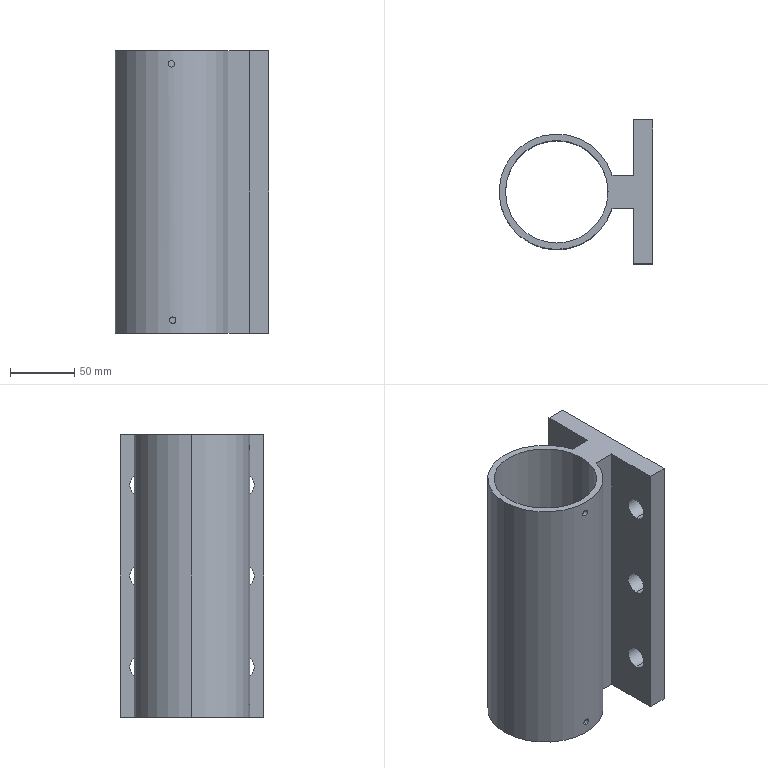Part | SolidWorks | features ICE 2, Extrusion 1 | 1 solid | 29 faces | box 120 x 112 x 220 mm | volume 732141 mm3 | cylinder 20 | plane 9 | commonest cylinder face diameters 17 x12 5 x4 80 x2 90 x2
STEP:
#1=CARTESIAN_POINT('',(0.,-45.,12.5));
#2=VERTEX_POINT('',#1);
#3=CARTESIAN_POINT('',(0.,-45.,7.5));
#4=VERTEX_POINT('',#3);
#5=CARTESIAN_POINT('',(0.,-45.,12.5));
#6=CARTESIAN_POINT('',(-0.1652,-45.,12.5));
#7=CARTESIAN_POINT('',(-0.3277,-44.999,12.484));
#8=CARTESIAN_POINT('',(-0.6473,-44.996,12.42));
#9=CARTESIAN_POINT('',(-0.806,-44.993,12.372));
#10=CARTESIAN_POINT('',(-1.109,-44.987,12.247));
#11=CARTESIAN_POINT('',(-1.252,-44.983,12.17));
#12=CARTESIAN_POINT('',(-1.524,-44.974,11.988));
#13=CARTESIAN_POINT('',(-1.653,-44.97,11.883));
#14=CARTESIAN_POINT('',(-1.883,-44.961,11.652));
#15=CARTESIAN_POINT('',(-1.987,-44.956,11.526));
#16=CARTESIAN_POINT('',(-2.17,-44.948,11.253));
#17=CARTESIAN_POINT('',(-2.247,-44.944,11.107));
#18=CARTESIAN_POINT('',(-2.372,-44.937,10.807));
#19=CARTESIAN_POINT('',(-2.42,-44.935,10.649));
#20=CARTESIAN_POINT('',(-2.484,-44.931,10.326));
#21=CARTESIAN_POINT('',(-2.5,-44.931,10.164));
#22=CARTESIAN_POINT('',(-2.5,-44.93,9.838));
#23=CARTESIAN_POINT('',(-2.484,-44.931,9.672));
#24=CARTESIAN_POINT('',(-2.42,-44.935,9.351));
#25=CARTESIAN_POINT('',(-2.373,-44.937,9.196));
#26=CARTESIAN_POINT('',(-2.247,-44.944,8.893));
#27=CARTESIAN_POINT('',(-2.169,-44.948,8.747));
#28=CARTESIAN_POINT('',(-1.988,-44.956,8.476));
#29=CARTESIAN_POINT('',(-1.885,-44.961,8.349));
#30=CARTESIAN_POINT('',(-1.651,-44.97,8.116));
#31=CARTESIAN_POINT('',(-1.525,-44.974,8.012));
#32=CARTESIAN_POINT('',(-1.254,-44.983,7.831));
#33=CARTESIAN_POINT('',(-1.108,-44.987,7.753));
#34=CARTESIAN_POINT('',(-0.8052,-44.993,7.628));
#35=CARTESIAN_POINT('',(-0.6493,-44.996,7.58));
#36=CARTESIAN_POINT('',(-0.3289,-44.999,7.516));
#37=CARTESIAN_POINT('',(-0.1632,-45.,7.5));
#38=CARTESIAN_POINT('',(0.,-45.,7.5));
#39=B_SPLINE_CURVE_WITH_KNOTS('',3,(#5,#6,#7,#8,#9,#10,#11,#12,#13,#14,#15,#16,#17,#18,#19,#20,#21,#22,#23,#24,#25,#26,#27,#28,#29,#30,#31,#32,#33,#34,#35,#36,#37,#38),.UNSPECIFIED.,.F.,.F.,(4,2,2,2,2,2,2,2,2,2,2,2,2,2,2,2,4),(0.,0.0004886,0.0009772,0.001466,0.001954,0.002443,0.002932,0.00342,0.003909,0.004397,0.004886,0.005375,0.005863,0.006352,0.00684,0.007329,0.007818),.UNSPECIFIED.);
#40=EDGE_CURVE('',#2,#4,#39,.T.);
#41=ORIENTED_EDGE('',*,*,#40,.T.);
#42=CARTESIAN_POINT('',(0.,-40.,7.5));
#43=VERTEX_POINT('',#42);
#44=CARTESIAN_POINT('',(0.,-56.001,7.5));
#45=DIRECTION('',(0.,1.,0.));
#46=VECTOR('',#45,1000.);
#47=LINE('',#44,#46);
#48=EDGE_CURVE('',#4,#43,#47,.T.);
#49=ORIENTED_EDGE('',*,*,#48,.T.);
#50=CARTESIAN_POINT('',(0.,-40.,12.5));
#51=VERTEX_POINT('',#50);
#52=CARTESIAN_POINT('',(0.,-40.,12.5));
#53=CARTESIAN_POINT('',(-0.1652,-40.,12.5));
#54=CARTESIAN_POINT('',(-0.3277,-39.999,12.484));
#55=CARTESIAN_POINT('',(-0.6473,-39.995,12.42));
#56=CARTESIAN_POINT('',(-0.8061,-39.992,12.372));
#57=CARTESIAN_POINT('',(-1.109,-39.985,12.247));
#58=CARTESIAN_POINT('',(-1.252,-39.981,12.17));
#59=CARTESIAN_POINT('',(-1.524,-39.971,11.988));
#60=CARTESIAN_POINT('',(-1.653,-39.966,11.883));
#61=CARTESIAN_POINT('',(-1.883,-39.956,11.652));
#62=CARTESIAN_POINT('',(-1.987,-39.951,11.526));
#63=CARTESIAN_POINT('',(-2.17,-39.941,11.253));
#64=CARTESIAN_POINT('',(-2.247,-39.937,11.107));
#65=CARTESIAN_POINT('',(-2.372,-39.93,10.807));
#66=CARTESIAN_POINT('',(-2.42,-39.927,10.649));
#67=CARTESIAN_POINT('',(-2.484,-39.923,10.326));
#68=CARTESIAN_POINT('',(-2.5,-39.922,10.164));
#69=CARTESIAN_POINT('',(-2.5,-39.922,9.838));
#70=CARTESIAN_POINT('',(-2.484,-39.923,9.672));
#71=CARTESIAN_POINT('',(-2.42,-39.927,9.351));
#72=CARTESIAN_POINT('',(-2.373,-39.93,9.196));
#73=CARTESIAN_POINT('',(-2.247,-39.937,8.893));
#74=CARTESIAN_POINT('',(-2.169,-39.941,8.746));
#75=CARTESIAN_POINT('',(-1.988,-39.951,8.476));
#76=CARTESIAN_POINT('',(-1.885,-39.956,8.349));
#77=CARTESIAN_POINT('',(-1.651,-39.966,8.116));
#78=CARTESIAN_POINT('',(-1.525,-39.971,8.012));
#79=CARTESIAN_POINT('',(-1.254,-39.981,7.831));
#80=CARTESIAN_POINT('',(-1.108,-39.985,7.753));
#81=CARTESIAN_POINT('',(-0.8052,-39.992,7.628));
#82=CARTESIAN_POINT('',(-0.6493,-39.995,7.58));
#83=CARTESIAN_POINT('',(-0.3289,-39.999,7.516));
#84=CARTESIAN_POINT('',(-0.1632,-40.,7.5));
#85=CARTESIAN_POINT('',(0.,-40.,7.5));
#86=B_SPLINE_CURVE_WITH_KNOTS('',3,(#52,#53,#54,#55,#56,#57,#58,#59,#60,#61,#62,#63,#64,#65,#66,#67,#68,#69,#70,#71,#72,#73,#74,#75,#76,#77,#78,#79,#80,#81,#82,#83,#84,#85),.UNSPECIFIED.,.F.,.F.,(4,2,2,2,2,2,2,2,2,2,2,2,2,2,2,2,4),(0.,0.0004886,0.0009773,0.001466,0.001955,0.002443,0.002932,0.00342,0.003909,0.004398,0.004886,0.005375,0.005864,0.006352,0.006841,0.007329,0.007818),.UNSPECIFIED.);
#87=EDGE_CURVE('',#51,#43,#86,.T.);
#88=ORIENTED_EDGE('',*,*,#87,.F.);
#89=CARTESIAN_POINT('',(0.,-56.001,12.5));
#90=DIRECTION('',(0.,1.,0.));
#91=VECTOR('',#90,1000.);
#92=LINE('',#89,#91);
#93=EDGE_CURVE('',#2,#51,#92,.T.);
#94=ORIENTED_EDGE('',*,*,#93,.F.);
#95=EDGE_LOOP('',(#41,#49,#88,#94));
#96=FACE_OUTER_BOUND('',#95,.T.);
#97=CARTESIAN_POINT('',(0.,-56.001,10.));
#98=DIRECTION('',(0.,1.,0.));
#99=DIRECTION('',(0.,0.,1.));
#100=AXIS2_PLACEMENT_3D('',#97,#98,#99);
#101=CYLINDRICAL_SURFACE('',#100,2.5);
#102=ADVANCED_FACE('',(#96),#101,.F.);
#103=CARTESIAN_POINT('',(-0.9593,-44.99,212.5));
#104=VERTEX_POINT('',#103);
#105=CARTESIAN_POINT('',(-0.9593,-44.99,207.5));
#106=VERTEX_POINT('',#105);
#107=CARTESIAN_POINT('',(-0.9593,-44.99,212.5));
#108=CARTESIAN_POINT('',(-1.125,-44.986,212.5));
#109=CARTESIAN_POINT('',(-1.287,-44.982,212.484));
#110=CARTESIAN_POINT('',(-1.607,-44.972,212.42));
#111=CARTESIAN_POINT('',(-1.765,-44.966,212.372));
#112=CARTESIAN_POINT('',(-2.068,-44.953,212.247));
#113=CARTESIAN_POINT('',(-2.212,-44.946,212.17));
#114=CARTESIAN_POINT('',(-2.483,-44.932,211.989));
#115=CARTESIAN_POINT('',(-2.612,-44.924,211.883));
#116=CARTESIAN_POINT('',(-2.843,-44.91,211.652));
#117=CARTESIAN_POINT('',(-2.946,-44.904,211.527));
#118=CARTESIAN_POINT('',(-3.129,-44.891,211.253));
#119=CARTESIAN_POINT('',(-3.206,-44.886,211.108));
#120=CARTESIAN_POINT('',(-3.331,-44.877,210.807));
#121=CARTESIAN_POINT('',(-3.379,-44.873,210.649));
#122=CARTESIAN_POINT('',(-3.443,-44.868,210.326));
#123=CARTESIAN_POINT('',(-3.459,-44.867,210.164));
#124=CARTESIAN_POINT('',(-3.459,-44.867,209.838));
#125=CARTESIAN_POINT('',(-3.443,-44.868,209.672));
#126=CARTESIAN_POINT('',(-3.379,-44.873,209.351));
#127=CARTESIAN_POINT('',(-3.332,-44.877,209.195));
#128=CARTESIAN_POINT('',(-3.207,-44.886,208.893));
#129=CARTESIAN_POINT('',(-3.128,-44.891,208.746));
#130=CARTESIAN_POINT('',(-2.947,-44.903,208.475));
#131=CARTESIAN_POINT('',(-2.844,-44.91,208.349));
#132=CARTESIAN_POINT('',(-2.611,-44.924,208.116));
#133=CARTESIAN_POINT('',(-2.484,-44.932,208.012));
#134=CARTESIAN_POINT('',(-2.213,-44.946,207.831));
#135=CARTESIAN_POINT('',(-2.067,-44.953,207.753));
#136=CARTESIAN_POINT('',(-1.764,-44.966,207.628));
#137=CARTESIAN_POINT('',(-1.609,-44.972,207.58));
#138=CARTESIAN_POINT('',(-1.288,-44.982,207.516));
#139=CARTESIAN_POINT('',(-1.123,-44.986,207.5));
#140=CARTESIAN_POINT('',(-0.9593,-44.99,207.5));
#141=B_SPLINE_CURVE_WITH_KNOTS('',3,(#107,#108,#109,#110,#111,#112,#113,#114,#115,#116,#117,#118,#119,#120,#121,#122,#123,#124,#125,#126,#127,#128,#129,#130,#131,#132,#133,#134,#135,#136,#137,#138,#139,#140),.UNSPECIFIED.,.F.,.F.,(4,2,2,2,2,2,2,2,2,2,2,2,2,2,2,2,4),(0.,0.0004888,0.0009776,0.001466,0.001955,0.002444,0.002933,0.003421,0.00391,0.004399,0.004888,0.005377,0.005865,0.006354,0.006843,0.007332,0.00782),.UNSPECIFIED.);
#142=EDGE_CURVE('',#104,#106,#141,.T.);
#143=ORIENTED_EDGE('',*,*,#142,.T.);
#144=CARTESIAN_POINT('',(-0.9593,-39.988,207.5));
#145=VERTEX_POINT('',#144);
#146=CARTESIAN_POINT('',(-0.9593,-56.001,207.5));
#147=DIRECTION('',(0.,1.,0.));
#148=VECTOR('',#147,1000.);
#149=LINE('',#146,#148);
#150=EDGE_CURVE('',#106,#145,#149,.T.);
#151=ORIENTED_EDGE('',*,*,#150,.T.);
#152=CARTESIAN_POINT('',(-0.9593,-39.988,212.5));
#153=VERTEX_POINT('',#152);
#154=CARTESIAN_POINT('',(-0.9593,-39.988,212.5));
#155=CARTESIAN_POINT('',(-1.125,-39.985,212.5));
#156=CARTESIAN_POINT('',(-1.287,-39.98,212.484));
#157=CARTESIAN_POINT('',(-1.607,-39.968,212.42));
#158=CARTESIAN_POINT('',(-1.765,-39.961,212.372));
#159=CARTESIAN_POINT('',(-2.068,-39.947,212.247));
#160=CARTESIAN_POINT('',(-2.212,-39.939,212.17));
#161=CARTESIAN_POINT('',(-2.483,-39.923,211.989));
#162=CARTESIAN_POINT('',(-2.612,-39.915,211.883));
#163=CARTESIAN_POINT('',(-2.842,-39.899,211.652));
#164=CARTESIAN_POINT('',(-2.946,-39.891,211.527));
#165=CARTESIAN_POINT('',(-3.129,-39.878,211.253));
#166=CARTESIAN_POINT('',(-3.206,-39.871,211.108));
#167=CARTESIAN_POINT('',(-3.331,-39.861,210.807));
#168=CARTESIAN_POINT('',(-3.379,-39.857,210.649));
#169=CARTESIAN_POINT('',(-3.443,-39.852,210.326));
#170=CARTESIAN_POINT('',(-3.459,-39.85,210.164));
#171=CARTESIAN_POINT('',(-3.459,-39.85,209.838));
#172=CARTESIAN_POINT('',(-3.443,-39.852,209.672));
#173=CARTESIAN_POINT('',(-3.379,-39.857,209.351));
#174=CARTESIAN_POINT('',(-3.332,-39.861,209.195));
#175=CARTESIAN_POINT('',(-3.207,-39.871,208.892));
#176=CARTESIAN_POINT('',(-3.128,-39.878,208.746));
#177=CARTESIAN_POINT('',(-2.947,-39.891,208.475));
#178=CARTESIAN_POINT('',(-2.844,-39.899,208.349));
#179=CARTESIAN_POINT('',(-2.611,-39.915,208.116));
#180=CARTESIAN_POINT('',(-2.484,-39.923,208.012));
#181=CARTESIAN_POINT('',(-2.213,-39.939,207.831));
#182=CARTESIAN_POINT('',(-2.067,-39.947,207.753));
#183=CARTESIAN_POINT('',(-1.765,-39.961,207.628));
#184=CARTESIAN_POINT('',(-1.609,-39.968,207.58));
#185=CARTESIAN_POINT('',(-1.288,-39.98,207.516));
#186=CARTESIAN_POINT('',(-1.123,-39.985,207.5));
#187=CARTESIAN_POINT('',(-0.9593,-39.988,207.5));
#188=B_SPLINE_CURVE_WITH_KNOTS('',3,(#154,#155,#156,#157,#158,#159,#160,#161,#162,#163,#164,#165,#166,#167,#168,#169,#170,#171,#172,#173,#174,#175,#176,#177,#178,#179,#180,#181,#182,#183,#184,#185,#186,#187),.UNSPECIFIED.,.F.,.F.,(4,2,2,2,2,2,2,2,2,2,2,2,2,2,2,2,4),(0.,0.0004888,0.0009777,0.001467,0.001955,0.002444,0.002933,0.003422,0.003911,0.0044,0.004888,0.005377,0.005866,0.006355,0.006844,0.007333,0.007822),.UNSPECIFIED.);
#189=EDGE_CURVE('',#153,#145,#188,.T.);
#190=ORIENTED_EDGE('',*,*,#189,.F.);
#191=CARTESIAN_POINT('',(-0.9593,-56.001,212.5));
#192=DIRECTION('',(0.,1.,0.));
#193=VECTOR('',#192,1000.);
#194=LINE('',#191,#193);
#195=EDGE_CURVE('',#104,#153,#194,.T.);
#196=ORIENTED_EDGE('',*,*,#195,.F.);
#197=EDGE_LOOP('',(#143,#151,#190,#196));
#198=FACE_OUTER_BOUND('',#197,.T.);
#199=CARTESIAN_POINT('',(-0.9593,-56.001,210.));
#200=DIRECTION('',(0.,1.,0.));
#201=DIRECTION('',(0.,0.,1.));
#202=AXIS2_PLACEMENT_3D('',#199,#200,#201);
#203=CYLINDRICAL_SURFACE('',#202,2.5);
#204=ADVANCED_FACE('',(#198),#203,.F.);
#205=CARTESIAN_POINT('',(60.,-40.,101.5));
#206=VERTEX_POINT('',#205);
#207=CARTESIAN_POINT('',(60.,-40.,118.5));
#208=VERTEX_POINT('',#207);
#209=CARTESIAN_POINT('',(60.,-40.,110.));
#210=DIRECTION('',(-1.,0.,0.));
#211=DIRECTION('',(0.,1.,0.));
#212=AXIS2_PLACEMENT_3D('',#209,#210,#211);
#213=CIRCLE('',#212,8.5);
#214=EDGE_CURVE('',#206,#208,#213,.T.);
#215=ORIENTED_EDGE('',*,*,#214,.T.);
#216=CARTESIAN_POINT('',(75.,-40.,118.5));
#217=VERTEX_POINT('',#216);
#218=CARTESIAN_POINT('',(-45.001,-40.,118.5));
#219=DIRECTION('',(1.,0.,0.));
#220=VECTOR('',#219,1000.);
#221=LINE('',#218,#220);
#222=EDGE_CURVE('',#208,#217,#221,.T.);
#223=ORIENTED_EDGE('',*,*,#222,.T.);
#224=CARTESIAN_POINT('',(75.,-40.,101.5));
#225=VERTEX_POINT('',#224);
#226=CARTESIAN_POINT('',(75.,-40.,110.));
#227=DIRECTION('',(1.,0.,0.));
#228=DIRECTION('',(0.,0.,-1.));
#229=AXIS2_PLACEMENT_3D('',#226,#227,#228);
#230=CIRCLE('',#229,8.5);
#231=EDGE_CURVE('',#217,#225,#230,.T.);
#232=ORIENTED_EDGE('',*,*,#231,.T.);
#233=CARTESIAN_POINT('',(-45.001,-40.,101.5));
#234=DIRECTION('',(1.,0.,0.));
#235=VECTOR('',#234,1000.);
#236=LINE('',#233,#235);
#237=EDGE_CURVE('',#206,#225,#236,.T.);
#238=ORIENTED_EDGE('',*,*,#237,.F.);
#239=EDGE_LOOP('',(#215,#223,#232,#238));
#240=FACE_OUTER_BOUND('',#239,.T.);
#241=CARTESIAN_POINT('',(-45.001,-40.,110.));
#242=DIRECTION('',(1.,0.,0.));
#243=DIRECTION('',(0.,0.,-1.));
#244=AXIS2_PLACEMENT_3D('',#241,#242,#243);
#245=CYLINDRICAL_SURFACE('',#244,8.5);
#246=ADVANCED_FACE('',(#240),#245,.F.);
#247=CARTESIAN_POINT('',(60.,-40.,30.5));
#248=VERTEX_POINT('',#247);
#249=CARTESIAN_POINT('',(60.,-40.,47.5));
#250=VERTEX_POINT('',#249);
#251=CARTESIAN_POINT('',(60.,-40.,39.));
#252=DIRECTION('',(-1.,0.,0.));
#253=DIRECTION('',(0.,1.,0.));
#254=AXIS2_PLACEMENT_3D('',#251,#252,#253);
#255=CIRCLE('',#254,8.5);
#256=EDGE_CURVE('',#248,#250,#255,.T.);
#257=ORIENTED_EDGE('',*,*,#256,.T.);
#258=CARTESIAN_POINT('',(75.,-40.,47.5));
#259=VERTEX_POINT('',#258);
#260=CARTESIAN_POINT('',(-45.001,-40.,47.5));
#261=DIRECTION('',(1.,0.,0.));
#262=VECTOR('',#261,1000.);
#263=LINE('',#260,#262);
#264=EDGE_CURVE('',#250,#259,#263,.T.);
#265=ORIENTED_EDGE('',*,*,#264,.T.);
#266=CARTESIAN_POINT('',(75.,-40.,30.5));
#267=VERTEX_POINT('',#266);
#268=CARTESIAN_POINT('',(75.,-40.,39.));
#269=DIRECTION('',(1.,0.,0.));
#270=DIRECTION('',(0.,0.,-1.));
#271=AXIS2_PLACEMENT_3D('',#268,#269,#270);
#272=CIRCLE('',#271,8.5);
#273=EDGE_CURVE('',#259,#267,#272,.T.);
#274=ORIENTED_EDGE('',*,*,#273,.T.);
#275=CARTESIAN_POINT('',(-45.001,-40.,30.5));
#276=DIRECTION('',(1.,0.,0.));
#277=VECTOR('',#276,1000.);
#278=LINE('',#275,#277);
#279=EDGE_CURVE('',#248,#267,#278,.T.);
#280=ORIENTED_EDGE('',*,*,#279,.F.);
#281=EDGE_LOOP('',(#257,#265,#274,#280));
#282=FACE_OUTER_BOUND('',#281,.T.);
#283=CARTESIAN_POINT('',(-45.001,-40.,39.));
#284=DIRECTION('',(1.,0.,0.));
#285=DIRECTION('',(0.,0.,-1.));
#286=AXIS2_PLACEMENT_3D('',#283,#284,#285);
#287=CYLINDRICAL_SURFACE('',#286,8.5);
#288=ADVANCED_FACE('',(#282),#287,.F.);
#289=CARTESIAN_POINT('',(60.,-40.,172.5));
#290=VERTEX_POINT('',#289);
#291=CARTESIAN_POINT('',(60.,-40.,189.5));
#292=VERTEX_POINT('',#291);
#293=CARTESIAN_POINT('',(60.,-40.,181.));
#294=DIRECTION('',(-1.,0.,0.));
#295=DIRECTION('',(0.,1.,0.));
#296=AXIS2_PLACEMENT_3D('',#293,#294,#295);
#297=CIRCLE('',#296,8.5);
#298=EDGE_CURVE('',#290,#292,#297,.T.);
#299=ORIENTED_EDGE('',*,*,#298,.T.);
#300=CARTESIAN_POINT('',(75.,-40.,189.5));
#301=VERTEX_POINT('',#300);
#302=CARTESIAN_POINT('',(-45.001,-40.,189.5));
#303=DIRECTION('',(1.,0.,0.));
#304=VECTOR('',#303,1000.);
#305=LINE('',#302,#304);
#306=EDGE_CURVE('',#292,#301,#305,.T.);
#307=ORIENTED_EDGE('',*,*,#306,.T.);
#308=CARTESIAN_POINT('',(75.,-40.,172.5));
#309=VERTEX_POINT('',#308);
#310=CARTESIAN_POINT('',(75.,-40.,181.));
#311=DIRECTION('',(1.,0.,0.));
#312=DIRECTION('',(0.,0.,-1.));
#313=AXIS2_PLACEMENT_3D('',#310,#311,#312);
#314=CIRCLE('',#313,8.5);
#315=EDGE_CURVE('',#301,#309,#314,.T.);
#316=ORIENTED_EDGE('',*,*,#315,.T.);
#317=CARTESIAN_POINT('',(-45.001,-40.,172.5));
#318=DIRECTION('',(1.,0.,0.));
#319=VECTOR('',#318,1000.);
#320=LINE('',#317,#319);
#321=EDGE_CURVE('',#290,#309,#320,.T.);
#322=ORIENTED_EDGE('',*,*,#321,.F.);
#323=EDGE_LOOP('',(#299,#307,#316,#322));
#324=FACE_OUTER_BOUND('',#323,.T.);
#325=CARTESIAN_POINT('',(-45.001,-40.,181.));
#326=DIRECTION('',(1.,0.,0.));
#327=DIRECTION('',(0.,0.,-1.));
#328=AXIS2_PLACEMENT_3D('',#325,#326,#327);
#329=CYLINDRICAL_SURFACE('',#328,8.5);
#330=ADVANCED_FACE('',(#324),#329,.F.);
#331=CARTESIAN_POINT('',(60.,40.,172.5));
#332=VERTEX_POINT('',#331);
#333=CARTESIAN_POINT('',(60.,40.,189.5));
#334=VERTEX_POINT('',#333);
#335=CARTESIAN_POINT('',(60.,40.,181.));
#336=DIRECTION('',(-1.,0.,0.));
#337=DIRECTION('',(0.,1.,0.));
#338=AXIS2_PLACEMENT_3D('',#335,#336,#337);
#339=CIRCLE('',#338,8.5);
#340=EDGE_CURVE('',#332,#334,#339,.T.);
#341=ORIENTED_EDGE('',*,*,#340,.T.);
#342=CARTESIAN_POINT('',(75.,40.,189.5));
#343=VERTEX_POINT('',#342);
#344=CARTESIAN_POINT('',(-45.001,40.,189.5));
#345=DIRECTION('',(1.,0.,0.));
#346=VECTOR('',#345,1000.);
#347=LINE('',#344,#346);
#348=EDGE_CURVE('',#334,#343,#347,.T.);
#349=ORIENTED_EDGE('',*,*,#348,.T.);
#350=CARTESIAN_POINT('',(75.,40.,172.5));
#351=VERTEX_POINT('',#350);
#352=CARTESIAN_POINT('',(75.,40.,181.));
#353=DIRECTION('',(1.,0.,0.));
#354=DIRECTION('',(0.,0.,-1.));
#355=AXIS2_PLACEMENT_3D('',#352,#353,#354);
#356=CIRCLE('',#355,8.5);
#357=EDGE_CURVE('',#343,#351,#356,.T.);
#358=ORIENTED_EDGE('',*,*,#357,.T.);
#359=CARTESIAN_POINT('',(-45.001,40.,172.5));
#360=DIRECTION('',(1.,0.,0.));
#361=VECTOR('',#360,1000.);
#362=LINE('',#359,#361);
#363=EDGE_CURVE('',#332,#351,#362,.T.);
#364=ORIENTED_EDGE('',*,*,#363,.F.);
#365=EDGE_LOOP('',(#341,#349,#358,#364));
#366=FACE_OUTER_BOUND('',#365,.T.);
#367=CARTESIAN_POINT('',(-45.001,40.,181.));
#368=DIRECTION('',(1.,0.,0.));
#369=DIRECTION('',(0.,0.,-1.));
#370=AXIS2_PLACEMENT_3D('',#367,#368,#369);
#371=CYLINDRICAL_SURFACE('',#370,8.5);
#372=ADVANCED_FACE('',(#366),#371,.F.);
#373=CARTESIAN_POINT('',(60.,40.,101.5));
#374=VERTEX_POINT('',#373);
#375=CARTESIAN_POINT('',(60.,40.,118.5));
#376=VERTEX_POINT('',#375);
#377=CARTESIAN_POINT('',(60.,40.,110.));
#378=DIRECTION('',(-1.,0.,0.));
#379=DIRECTION('',(0.,1.,0.));
#380=AXIS2_PLACEMENT_3D('',#377,#378,#379);
#381=CIRCLE('',#380,8.5);
#382=EDGE_CURVE('',#374,#376,#381,.T.);
#383=ORIENTED_EDGE('',*,*,#382,.T.);
#384=CARTESIAN_POINT('',(75.,40.,118.5));
#385=VERTEX_POINT('',#384);
#386=CARTESIAN_POINT('',(-45.001,40.,118.5));
#387=DIRECTION('',(1.,0.,0.));
#388=VECTOR('',#387,1000.);
#389=LINE('',#386,#388);
#390=EDGE_CURVE('',#376,#385,#389,.T.);
#391=ORIENTED_EDGE('',*,*,#390,.T.);
#392=CARTESIAN_POINT('',(75.,40.,101.5));
#393=VERTEX_POINT('',#392);
#394=CARTESIAN_POINT('',(75.,40.,110.));
#395=DIRECTION('',(1.,0.,0.));
#396=DIRECTION('',(0.,0.,-1.));
#397=AXIS2_PLACEMENT_3D('',#394,#395,#396);
#398=CIRCLE('',#397,8.5);
#399=EDGE_CURVE('',#385,#393,#398,.T.);
#400=ORIENTED_EDGE('',*,*,#399,.T.);
#401=CARTESIAN_POINT('',(-45.001,40.,101.5));
#402=DIRECTION('',(1.,0.,0.));
#403=VECTOR('',#402,1000.);
#404=LINE('',#401,#403);
#405=EDGE_CURVE('',#374,#393,#404,.T.);
#406=ORIENTED_EDGE('',*,*,#405,.F.);
#407=EDGE_LOOP('',(#383,#391,#400,#406));
#408=FACE_OUTER_BOUND('',#407,.T.);
#409=CARTESIAN_POINT('',(-45.001,40.,110.));
#410=DIRECTION('',(1.,0.,0.));
#411=DIRECTION('',(0.,0.,-1.));
#412=AXIS2_PLACEMENT_3D('',#409,#410,#411);
#413=CYLINDRICAL_SURFACE('',#412,8.5);
#414=ADVANCED_FACE('',(#408),#413,.F.);
#415=CARTESIAN_POINT('',(60.,40.,30.5));
#416=VERTEX_POINT('',#415);
#417=CARTESIAN_POINT('',(60.,40.,47.5));
#418=VERTEX_POINT('',#417);
#419=CARTESIAN_POINT('',(60.,40.,39.));
#420=DIRECTION('',(-1.,0.,0.));
#421=DIRECTION('',(0.,1.,0.));
#422=AXIS2_PLACEMENT_3D('',#419,#420,#421);
#423=CIRCLE('',#422,8.5);
#424=EDGE_CURVE('',#416,#418,#423,.T.);
#425=ORIENTED_EDGE('',*,*,#424,.T.);
#426=CARTESIAN_POINT('',(75.,40.,47.5));
#427=VERTEX_POINT('',#426);
#428=CARTESIAN_POINT('',(-45.001,40.,47.5));
#429=DIRECTION('',(1.,0.,0.));
#430=VECTOR('',#429,1000.);
#431=LINE('',#428,#430);
#432=EDGE_CURVE('',#418,#427,#431,.T.);
#433=ORIENTED_EDGE('',*,*,#432,.T.);
#434=CARTESIAN_POINT('',(75.,40.,30.5));
#435=VERTEX_POINT('',#434);
#436=CARTESIAN_POINT('',(75.,40.,39.));
#437=DIRECTION('',(1.,0.,0.));
#438=DIRECTION('',(0.,0.,-1.));
#439=AXIS2_PLACEMENT_3D('',#436,#437,#438);
#440=CIRCLE('',#439,8.5);
#441=EDGE_CURVE('',#427,#435,#440,.T.);
#442=ORIENTED_EDGE('',*,*,#441,.T.);
#443=CARTESIAN_POINT('',(-45.001,40.,30.5));
#444=DIRECTION('',(1.,0.,0.));
#445=VECTOR('',#444,1000.);
#446=LINE('',#443,#445);
#447=EDGE_CURVE('',#416,#435,#446,.T.);
#448=ORIENTED_EDGE('',*,*,#447,.F.);
#449=EDGE_LOOP('',(#425,#433,#442,#448));
#450=FACE_OUTER_BOUND('',#449,.T.);
#451=CARTESIAN_POINT('',(-45.001,40.,39.));
#452=DIRECTION('',(1.,0.,0.));
#453=DIRECTION('',(0.,0.,-1.));
#454=AXIS2_PLACEMENT_3D('',#451,#452,#453);
#455=CYLINDRICAL_SURFACE('',#454,8.5);
#456=ADVANCED_FACE('',(#450),#455,.F.);
#457=ORIENTED_EDGE('',*,*,#87,.T.);
#458=CARTESIAN_POINT('',(0.,-40.,7.5));
#459=CARTESIAN_POINT('',(0.1631,-40.,7.5));
#460=CARTESIAN_POINT('',(0.3253,-39.999,7.516));
#461=CARTESIAN_POINT('',(0.6477,-39.995,7.58));
#462=CARTESIAN_POINT('',(0.8056,-39.992,7.628));
#463=CARTESIAN_POINT('',(1.257,-39.981,7.815));
#464=CARTESIAN_POINT('',(1.536,-39.971,8.001));
#465=CARTESIAN_POINT('',(1.882,-39.956,8.346));
#466=CARTESIAN_POINT('',(1.987,-39.951,8.475));
#467=CARTESIAN_POINT('',(2.169,-39.941,8.746));
#468=CARTESIAN_POINT('',(2.246,-39.937,8.89));
#469=CARTESIAN_POINT('',(2.372,-39.93,9.192));
#470=CARTESIAN_POINT('',(2.42,-39.927,9.351));
#471=CARTESIAN_POINT('',(2.484,-39.923,9.671));
#472=CARTESIAN_POINT('',(2.5,-39.922,9.833));
#473=CARTESIAN_POINT('',(2.5,-39.922,10.163));
#474=CARTESIAN_POINT('',(2.484,-39.923,10.326));
#475=CARTESIAN_POINT('',(2.421,-39.927,10.645));
#476=CARTESIAN_POINT('',(2.373,-39.93,10.804));
#477=CARTESIAN_POINT('',(2.248,-39.937,11.107));
#478=CARTESIAN_POINT('',(2.171,-39.941,11.251));
#479=CARTESIAN_POINT('',(1.99,-39.951,11.522));
#480=CARTESIAN_POINT('',(1.884,-39.956,11.651));
#481=CARTESIAN_POINT('',(1.654,-39.966,11.882));
#482=CARTESIAN_POINT('',(1.528,-39.971,11.985));
#483=CARTESIAN_POINT('',(1.255,-39.981,12.168));
#484=CARTESIAN_POINT('',(1.11,-39.985,12.246));
#485=CARTESIAN_POINT('',(0.6586,-39.996,12.434));
#486=CARTESIAN_POINT('',(0.3304,-40.,12.5));
#487=CARTESIAN_POINT('',(0.,-40.,12.5));
#488=B_SPLINE_CURVE_WITH_KNOTS('',3,(#458,#459,#460,#461,#462,#463,#464,#465,#466,#467,#468,#469,#470,#471,#472,#473,#474,#475,#476,#477,#478,#479,#480,#481,#482,#483,#484,#485,#486,#487),.UNSPECIFIED.,.F.,.F.,(4,2,2,2,2,2,2,2,2,2,2,2,2,2,4),(0.007818,0.008307,0.008795,0.009772,0.01026,0.01075,0.01124,0.01173,0.01221,0.0127,0.01319,0.01368,0.01417,0.01466,0.01563),.UNSPECIFIED.);
#489=EDGE_CURVE('',#43,#51,#488,.T.);
#490=ORIENTED_EDGE('',*,*,#489,.T.);
#491=EDGE_LOOP('',(#457,#490));
#492=FACE_BOUND('',#491,.T.);
#493=ORIENTED_EDGE('',*,*,#189,.T.);
#494=CARTESIAN_POINT('',(-0.9593,-39.988,207.5));
#495=CARTESIAN_POINT('',(-0.7963,-39.992,207.5));
#496=CARTESIAN_POINT('',(-0.6342,-39.995,207.516));
#497=CARTESIAN_POINT('',(-0.3119,-39.999,207.58));
#498=CARTESIAN_POINT('',(-0.1539,-40.,207.628));
#499=CARTESIAN_POINT('',(0.2974,-40.,207.814));
#500=CARTESIAN_POINT('',(0.5765,-39.997,208.001));
#501=CARTESIAN_POINT('',(0.9225,-39.99,208.346));
#502=CARTESIAN_POINT('',(1.028,-39.987,208.475));
#503=CARTESIAN_POINT('',(1.21,-39.982,208.746));
#504=CARTESIAN_POINT('',(1.287,-39.979,208.89));
#505=CARTESIAN_POINT('',(1.412,-39.975,209.192));
#506=CARTESIAN_POINT('',(1.461,-39.973,209.351));
#507=CARTESIAN_POINT('',(1.524,-39.971,209.671));
#508=CARTESIAN_POINT('',(1.541,-39.97,209.833));
#509=CARTESIAN_POINT('',(1.541,-39.97,210.163));
#510=CARTESIAN_POINT('',(1.525,-39.971,210.326));
#511=CARTESIAN_POINT('',(1.461,-39.973,210.645));
#512=CARTESIAN_POINT('',(1.414,-39.975,210.804));
#513=CARTESIAN_POINT('',(1.288,-39.979,211.107));
#514=CARTESIAN_POINT('',(1.212,-39.982,211.251));
#515=CARTESIAN_POINT('',(1.03,-39.987,211.522));
#516=CARTESIAN_POINT('',(0.925,-39.989,211.651));
#517=CARTESIAN_POINT('',(0.6944,-39.994,211.882));
#518=CARTESIAN_POINT('',(0.5687,-39.996,211.985));
#519=CARTESIAN_POINT('',(0.2959,-39.999,212.168));
#520=CARTESIAN_POINT('',(0.1501,-40.,212.246));
#521=CARTESIAN_POINT('',(-0.301,-40.,212.434));
#522=CARTESIAN_POINT('',(-0.6291,-39.996,212.5));
#523=CARTESIAN_POINT('',(-0.9593,-39.988,212.5));
#524=B_SPLINE_CURVE_WITH_KNOTS('',3,(#494,#495,#496,#497,#498,#499,#500,#501,#502,#503,#504,#505,#506,#507,#508,#509,#510,#511,#512,#513,#514,#515,#516,#517,#518,#519,#520,#521,#522,#523),.UNSPECIFIED.,.F.,.F.,(4,2,2,2,2,2,2,2,2,2,2,2,2,2,4),(0.007822,0.00831,0.008798,0.009775,0.01026,0.01075,0.01124,0.01173,0.01222,0.01271,0.01319,0.01368,0.01417,0.01466,0.01564),.UNSPECIFIED.);
#525=EDGE_CURVE('',#145,#153,#524,.T.);
#526=ORIENTED_EDGE('',*,*,#525,.T.);
#527=EDGE_LOOP('',(#493,#526));
#528=FACE_BOUND('',#527,.T.);
#529=CARTESIAN_POINT('',(-40.,0.,220.));
#530=VERTEX_POINT('',#529);
#531=CARTESIAN_POINT('',(40.,0.,220.));
#532=VERTEX_POINT('',#531);
#533=CARTESIAN_POINT('',(0.,0.,220.));
#534=DIRECTION('',(0.,0.,1.));
#535=DIRECTION('',(1.,0.,0.));
#536=AXIS2_PLACEMENT_3D('',#533,#534,#535);
#537=CIRCLE('',#536,40.);
#538=EDGE_CURVE('',#530,#532,#537,.T.);
#539=ORIENTED_EDGE('',*,*,#538,.T.);
#540=CARTESIAN_POINT('',(40.,0.,0.));
#541=VERTEX_POINT('',#540);
#542=CARTESIAN_POINT('',(40.,0.,220.));
#543=DIRECTION('',(0.,0.,-1.));
#544=VECTOR('',#543,1000.);
#545=LINE('',#542,#544);
#546=EDGE_CURVE('',#532,#541,#545,.T.);
#547=ORIENTED_EDGE('',*,*,#546,.T.);
#548=CARTESIAN_POINT('',(-40.,0.,0.));
#549=VERTEX_POINT('',#548);
#550=CARTESIAN_POINT('',(0.,0.,0.));
#551=DIRECTION('',(0.,0.,1.));
#552=DIRECTION('',(1.,0.,0.));
#553=AXIS2_PLACEMENT_3D('',#550,#551,#552);
#554=CIRCLE('',#553,40.);
#555=EDGE_CURVE('',#549,#541,#554,.T.);
#556=ORIENTED_EDGE('',*,*,#555,.F.);
#557=CARTESIAN_POINT('',(-40.,0.,220.));
#558=DIRECTION('',(0.,0.,-1.));
#559=VECTOR('',#558,1000.);
#560=LINE('',#557,#559);
#561=EDGE_CURVE('',#530,#549,#560,.T.);
#562=ORIENTED_EDGE('',*,*,#561,.F.);
#563=EDGE_LOOP('',(#539,#547,#556,#562));
#564=FACE_OUTER_BOUND('',#563,.T.);
#565=CARTESIAN_POINT('',(0.,0.,220.));
#566=DIRECTION('',(0.,0.,-1.));
#567=DIRECTION('',(-1.,0.,0.));
#568=AXIS2_PLACEMENT_3D('',#565,#566,#567);
#569=CYLINDRICAL_SURFACE('',#568,40.);
#570=ADVANCED_FACE('',(#492,#528,#564),#569,.F.);
#571=ORIENTED_EDGE('',*,*,#40,.F.);
#572=CARTESIAN_POINT('',(0.,-45.,7.5));
#573=CARTESIAN_POINT('',(0.1631,-45.,7.5));
#574=CARTESIAN_POINT('',(0.3253,-44.999,7.516));
#575=CARTESIAN_POINT('',(0.6476,-44.996,7.58));
#576=CARTESIAN_POINT('',(0.8056,-44.993,7.628));
#577=CARTESIAN_POINT('',(1.257,-44.983,7.815));
#578=CARTESIAN_POINT('',(1.536,-44.974,8.001));
#579=CARTESIAN_POINT('',(1.882,-44.961,8.346));
#580=CARTESIAN_POINT('',(1.987,-44.956,8.475));
#581=CARTESIAN_POINT('',(2.169,-44.948,8.746));
#582=CARTESIAN_POINT('',(2.246,-44.944,8.89));
#583=CARTESIAN_POINT('',(2.372,-44.938,9.192));
#584=CARTESIAN_POINT('',(2.42,-44.935,9.351));
#585=CARTESIAN_POINT('',(2.484,-44.931,9.671));
#586=CARTESIAN_POINT('',(2.5,-44.931,9.833));
#587=CARTESIAN_POINT('',(2.5,-44.93,10.163));
#588=CARTESIAN_POINT('',(2.484,-44.931,10.326));
#589=CARTESIAN_POINT('',(2.421,-44.935,10.645));
#590=CARTESIAN_POINT('',(2.373,-44.937,10.804));
#591=CARTESIAN_POINT('',(2.248,-44.944,11.107));
#592=CARTESIAN_POINT('',(2.171,-44.948,11.251));
#593=CARTESIAN_POINT('',(1.99,-44.956,11.522));
#594=CARTESIAN_POINT('',(1.884,-44.961,11.651));
#595=CARTESIAN_POINT('',(1.654,-44.97,11.882));
#596=CARTESIAN_POINT('',(1.528,-44.974,11.985));
#597=CARTESIAN_POINT('',(1.255,-44.983,12.168));
#598=CARTESIAN_POINT('',(1.11,-44.987,12.246));
#599=CARTESIAN_POINT('',(0.6585,-44.996,12.434));
#600=CARTESIAN_POINT('',(0.3304,-45.,12.5));
#601=CARTESIAN_POINT('',(0.,-45.,12.5));
#602=B_SPLINE_CURVE_WITH_KNOTS('',3,(#572,#573,#574,#575,#576,#577,#578,#579,#580,#581,#582,#583,#584,#585,#586,#587,#588,#589,#590,#591,#592,#593,#594,#595,#596,#597,#598,#599,#600,#601),.UNSPECIFIED.,.F.,.F.,(4,2,2,2,2,2,2,2,2,2,2,2,2,2,4),(0.007818,0.008306,0.008795,0.009772,0.01026,0.01075,0.01124,0.01173,0.01221,0.0127,0.01319,0.01368,0.01417,0.01466,0.01563),.UNSPECIFIED.);
#603=EDGE_CURVE('',#4,#2,#602,.T.);
#604=ORIENTED_EDGE('',*,*,#603,.F.);
#605=EDGE_LOOP('',(#571,#604));
#606=FACE_BOUND('',#605,.T.);
#607=ORIENTED_EDGE('',*,*,#142,.F.);
#608=CARTESIAN_POINT('',(-0.9593,-44.99,207.5));
#609=CARTESIAN_POINT('',(-0.7963,-44.993,207.5));
#610=CARTESIAN_POINT('',(-0.6341,-44.996,207.516));
#611=CARTESIAN_POINT('',(-0.3119,-44.999,207.58));
#612=CARTESIAN_POINT('',(-0.1539,-45.,207.628));
#613=CARTESIAN_POINT('',(0.2974,-45.,207.814));
#614=CARTESIAN_POINT('',(0.5765,-44.997,208.001));
#615=CARTESIAN_POINT('',(0.9225,-44.991,208.346));
#616=CARTESIAN_POINT('',(1.028,-44.988,208.475));
#617=CARTESIAN_POINT('',(1.21,-44.984,208.746));
#618=CARTESIAN_POINT('',(1.287,-44.982,208.89));
#619=CARTESIAN_POINT('',(1.412,-44.978,209.192));
#620=CARTESIAN_POINT('',(1.461,-44.976,209.351));
#621=CARTESIAN_POINT('',(1.524,-44.974,209.671));
#622=CARTESIAN_POINT('',(1.541,-44.974,209.833));
#623=CARTESIAN_POINT('',(1.541,-44.974,210.163));
#624=CARTESIAN_POINT('',(1.525,-44.974,210.326));
#625=CARTESIAN_POINT('',(1.461,-44.976,210.645));
#626=CARTESIAN_POINT('',(1.414,-44.978,210.804));
#627=CARTESIAN_POINT('',(1.288,-44.982,211.107));
#628=CARTESIAN_POINT('',(1.212,-44.984,211.251));
#629=CARTESIAN_POINT('',(1.03,-44.988,211.522));
#630=CARTESIAN_POINT('',(0.925,-44.991,211.651));
#631=CARTESIAN_POINT('',(0.6944,-44.995,211.882));
#632=CARTESIAN_POINT('',(0.5687,-44.997,211.985));
#633=CARTESIAN_POINT('',(0.2959,-44.999,212.168));
#634=CARTESIAN_POINT('',(0.1501,-45.,212.246));
#635=CARTESIAN_POINT('',(-0.301,-45.,212.434));
#636=CARTESIAN_POINT('',(-0.6291,-44.997,212.5));
#637=CARTESIAN_POINT('',(-0.9593,-44.99,212.5));
#638=B_SPLINE_CURVE_WITH_KNOTS('',3,(#608,#609,#610,#611,#612,#613,#614,#615,#616,#617,#618,#619,#620,#621,#622,#623,#624,#625,#626,#627,#628,#629,#630,#631,#632,#633,#634,#635,#636,#637),.UNSPECIFIED.,.F.,.F.,(4,2,2,2,2,2,2,2,2,2,2,2,2,2,4),(0.00782,0.008309,0.008797,0.009774,0.01026,0.01075,0.01124,0.01173,0.01222,0.0127,0.01319,0.01368,0.01417,0.01466,0.01564),.UNSPECIFIED.);
#639=EDGE_CURVE('',#106,#104,#638,.T.);
#640=ORIENTED_EDGE('',*,*,#639,.F.);
#641=EDGE_LOOP('',(#607,#640));
#642=FACE_BOUND('',#641,.T.);
#643=CARTESIAN_POINT('',(-45.,0.,220.));
#644=VERTEX_POINT('',#643);
#645=CARTESIAN_POINT('',(43.081,-13.,220.));
#646=VERTEX_POINT('',#645);
#647=CARTESIAN_POINT('',(0.,0.,220.));
#648=DIRECTION('',(0.,0.,1.));
#649=DIRECTION('',(1.,0.,0.));
#650=AXIS2_PLACEMENT_3D('',#647,#648,#649);
#651=CIRCLE('',#650,45.);
#652=EDGE_CURVE('',#644,#646,#651,.T.);
#653=ORIENTED_EDGE('',*,*,#652,.F.);
#654=CARTESIAN_POINT('',(-45.,0.,0.));
#655=VERTEX_POINT('',#654);
#656=CARTESIAN_POINT('',(-45.,0.,220.));
#657=DIRECTION('',(0.,0.,-1.));
#658=VECTOR('',#657,1000.);
#659=LINE('',#656,#658);
#660=EDGE_CURVE('',#644,#655,#659,.T.);
#661=ORIENTED_EDGE('',*,*,#660,.T.);
#662=CARTESIAN_POINT('',(43.081,-13.,0.));
#663=VERTEX_POINT('',#662);
#664=CARTESIAN_POINT('',(0.,0.,0.));
#665=DIRECTION('',(0.,0.,1.));
#666=DIRECTION('',(1.,0.,0.));
#667=AXIS2_PLACEMENT_3D('',#664,#665,#666);
#668=CIRCLE('',#667,45.);
#669=EDGE_CURVE('',#655,#663,#668,.T.);
#670=ORIENTED_EDGE('',*,*,#669,.T.);
#671=CARTESIAN_POINT('',(43.081,-13.,220.));
#672=DIRECTION('',(0.,0.,-1.));
#673=VECTOR('',#672,1000.);
#674=LINE('',#671,#673);
#675=EDGE_CURVE('',#646,#663,#674,.T.);
#676=ORIENTED_EDGE('',*,*,#675,.F.);
#677=EDGE_LOOP('',(#653,#661,#670,#676));
#678=FACE_OUTER_BOUND('',#677,.T.);
#679=CARTESIAN_POINT('',(0.,0.,220.));
#680=DIRECTION('',(0.,0.,-1.));
#681=DIRECTION('',(-1.,0.,0.));
#682=AXIS2_PLACEMENT_3D('',#679,#680,#681);
#683=CYLINDRICAL_SURFACE('',#682,45.);
#684=ADVANCED_FACE('',(#606,#642,#678),#683,.T.);
#685=CARTESIAN_POINT('',(60.,-13.,220.));
#686=VERTEX_POINT('',#685);
#687=CARTESIAN_POINT('',(60.,-56.,220.));
#688=VERTEX_POINT('',#687);
#689=CARTESIAN_POINT('',(60.,-13.,220.));
#690=DIRECTION('',(0.,-1.,0.));
#691=VECTOR('',#690,1000.);
#692=LINE('',#689,#691);
#693=EDGE_CURVE('',#686,#688,#692,.T.);
#694=ORIENTED_EDGE('',*,*,#693,.T.);
#695=CARTESIAN_POINT('',(75.,-56.,220.));
#696=VERTEX_POINT('',#695);
#697=CARTESIAN_POINT('',(75.,-56.,220.));
#698=DIRECTION('',(1.,0.,0.));
#699=VECTOR('',#698,1000.);
#700=LINE('',#697,#699);
#701=EDGE_CURVE('',#688,#696,#700,.T.);
#702=ORIENTED_EDGE('',*,*,#701,.T.);
#703=CARTESIAN_POINT('',(75.,56.,220.));
#704=VERTEX_POINT('',#703);
#705=CARTESIAN_POINT('',(75.,56.,220.));
#706=DIRECTION('',(0.,1.,0.));
#707=VECTOR('',#706,1000.);
#708=LINE('',#705,#707);
#709=EDGE_CURVE('',#696,#704,#708,.T.);
#710=ORIENTED_EDGE('',*,*,#709,.T.);
#711=CARTESIAN_POINT('',(60.,56.,220.));
#712=VERTEX_POINT('',#711);
#713=CARTESIAN_POINT('',(75.,56.,220.));
#714=DIRECTION('',(-1.,0.,0.));
#715=VECTOR('',#714,1000.);
#716=LINE('',#713,#715);
#717=EDGE_CURVE('',#704,#712,#716,.T.);
#718=ORIENTED_EDGE('',*,*,#717,.T.);
#719=CARTESIAN_POINT('',(60.,13.,220.));
#720=VERTEX_POINT('',#719);
#721=CARTESIAN_POINT('',(60.,56.,220.));
#722=DIRECTION('',(0.,-1.,0.));
#723=VECTOR('',#722,1000.);
#724=LINE('',#721,#723);
#725=EDGE_CURVE('',#712,#720,#724,.T.);
#726=ORIENTED_EDGE('',*,*,#725,.T.);
#727=CARTESIAN_POINT('',(43.081,13.,220.));
#728=VERTEX_POINT('',#727);
#729=CARTESIAN_POINT('',(43.081,13.,220.));
#730=DIRECTION('',(-1.,0.,0.));
#731=VECTOR('',#730,1000.);
#732=LINE('',#729,#731);
#733=EDGE_CURVE('',#720,#728,#732,.T.);
#734=ORIENTED_EDGE('',*,*,#733,.T.);
#735=CARTESIAN_POINT('',(0.,0.,220.));
#736=DIRECTION('',(0.,0.,1.));
#737=DIRECTION('',(1.,0.,0.));
#738=AXIS2_PLACEMENT_3D('',#735,#736,#737);
#739=CIRCLE('',#738,45.);
#740=EDGE_CURVE('',#728,#644,#739,.T.);
#741=ORIENTED_EDGE('',*,*,#740,.T.);
#742=ORIENTED_EDGE('',*,*,#652,.T.);
#743=CARTESIAN_POINT('',(43.081,-13.,220.));
#744=DIRECTION('',(1.,0.,0.));
#745=VECTOR('',#744,1000.);
#746=LINE('',#743,#745);
#747=EDGE_CURVE('',#646,#686,#746,.T.);
#748=ORIENTED_EDGE('',*,*,#747,.T.);
#749=EDGE_LOOP('',(#694,#702,#710,#718,#726,#734,#741,#742,#748));
#750=FACE_OUTER_BOUND('',#749,.T.);
#751=ORIENTED_EDGE('',*,*,#538,.F.);
#752=CARTESIAN_POINT('',(0.,0.,220.));
#753=DIRECTION('',(0.,0.,1.));
#754=DIRECTION('',(1.,0.,0.));
#755=AXIS2_PLACEMENT_3D('',#752,#753,#754);
#756=CIRCLE('',#755,40.);
#757=EDGE_CURVE('',#532,#530,#756,.T.);
#758=ORIENTED_EDGE('',*,*,#757,.F.);
#759=EDGE_LOOP('',(#751,#758));
#760=FACE_BOUND('',#759,.T.);
#761=CARTESIAN_POINT('',(0.,0.,220.));
#762=DIRECTION('',(0.,0.,1.));
#763=DIRECTION('',(1.,0.,0.));
#764=AXIS2_PLACEMENT_3D('',#761,#762,#763);
#765=PLANE('',#764);
#766=ADVANCED_FACE('',(#750,#760),#765,.T.);
#767=CARTESIAN_POINT('',(60.,-13.,0.));
#768=VERTEX_POINT('',#767);
#769=CARTESIAN_POINT('',(60.,-56.,0.));
#770=VERTEX_POINT('',#769);
#771=CARTESIAN_POINT('',(60.,-13.,0.));
#772=DIRECTION('',(0.,-1.,0.));
#773=VECTOR('',#772,1000.);
#774=LINE('',#771,#773);
#775=EDGE_CURVE('',#768,#770,#774,.T.);
#776=ORIENTED_EDGE('',*,*,#775,.F.);
#777=CARTESIAN_POINT('',(43.081,-13.,0.));
#778=DIRECTION('',(1.,0.,0.));
#779=VECTOR('',#778,1000.);
#780=LINE('',#777,#779);
#781=EDGE_CURVE('',#663,#768,#780,.T.);
#782=ORIENTED_EDGE('',*,*,#781,.F.);
#783=ORIENTED_EDGE('',*,*,#669,.F.);
#784=CARTESIAN_POINT('',(43.081,13.,0.));
#785=VERTEX_POINT('',#784);
#786=CARTESIAN_POINT('',(0.,0.,0.));
#787=DIRECTION('',(0.,0.,1.));
#788=DIRECTION('',(1.,0.,0.));
#789=AXIS2_PLACEMENT_3D('',#786,#787,#788);
#790=CIRCLE('',#789,45.);
#791=EDGE_CURVE('',#785,#655,#790,.T.);
#792=ORIENTED_EDGE('',*,*,#791,.F.);
#793=CARTESIAN_POINT('',(60.,13.,0.));
#794=VERTEX_POINT('',#793);
#795=CARTESIAN_POINT('',(43.081,13.,0.));
#796=DIRECTION('',(-1.,0.,0.));
#797=VECTOR('',#796,1000.);
#798=LINE('',#795,#797);
#799=EDGE_CURVE('',#794,#785,#798,.T.);
#800=ORIENTED_EDGE('',*,*,#799,.F.);
#801=CARTESIAN_POINT('',(60.,56.,0.));
#802=VERTEX_POINT('',#801);
#803=CARTESIAN_POINT('',(60.,56.,0.));
#804=DIRECTION('',(0.,-1.,0.));
#805=VECTOR('',#804,1000.);
#806=LINE('',#803,#805);
#807=EDGE_CURVE('',#802,#794,#806,.T.);
#808=ORIENTED_EDGE('',*,*,#807,.F.);
#809=CARTESIAN_POINT('',(75.,56.,0.));
#810=VERTEX_POINT('',#809);
#811=CARTESIAN_POINT('',(75.,56.,0.));
#812=DIRECTION('',(-1.,0.,0.));
#813=VECTOR('',#812,1000.);
#814=LINE('',#811,#813);
#815=EDGE_CURVE('',#810,#802,#814,.T.);
#816=ORIENTED_EDGE('',*,*,#815,.F.);
#817=CARTESIAN_POINT('',(75.,-56.,0.));
#818=VERTEX_POINT('',#817);
#819=CARTESIAN_POINT('',(75.,56.,0.));
#820=DIRECTION('',(0.,1.,0.));
#821=VECTOR('',#820,1000.);
#822=LINE('',#819,#821);
#823=EDGE_CURVE('',#818,#810,#822,.T.);
#824=ORIENTED_EDGE('',*,*,#823,.F.);
#825=CARTESIAN_POINT('',(75.,-56.,0.));
#826=DIRECTION('',(1.,0.,0.));
#827=VECTOR('',#826,1000.);
#828=LINE('',#825,#827);
#829=EDGE_CURVE('',#770,#818,#828,.T.);
#830=ORIENTED_EDGE('',*,*,#829,.F.);
#831=EDGE_LOOP('',(#776,#782,#783,#792,#800,#808,#816,#824,#830));
#832=FACE_OUTER_BOUND('',#831,.T.);
#833=ORIENTED_EDGE('',*,*,#555,.T.);
#834=CARTESIAN_POINT('',(0.,0.,0.));
#835=DIRECTION('',(0.,0.,1.));
#836=DIRECTION('',(1.,0.,0.));
#837=AXIS2_PLACEMENT_3D('',#834,#835,#836);
#838=CIRCLE('',#837,40.);
#839=EDGE_CURVE('',#541,#549,#838,.T.);
#840=ORIENTED_EDGE('',*,*,#839,.T.);
#841=EDGE_LOOP('',(#833,#840));
#842=FACE_BOUND('',#841,.T.);
#843=CARTESIAN_POINT('',(0.,0.,0.));
#844=DIRECTION('',(0.,0.,1.));
#845=DIRECTION('',(1.,0.,0.));
#846=AXIS2_PLACEMENT_3D('',#843,#844,#845);
#847=PLANE('',#846);
#848=ADVANCED_FACE('',(#832,#842),#847,.F.);
#849=ORIENTED_EDGE('',*,*,#214,.F.);
#850=CARTESIAN_POINT('',(60.,-40.,110.));
#851=DIRECTION('',(-1.,0.,0.));
#852=DIRECTION('',(0.,1.,0.));
#853=AXIS2_PLACEMENT_3D('',#850,#851,#852);
#854=CIRCLE('',#853,8.5);
#855=EDGE_CURVE('',#208,#206,#854,.T.);
#856=ORIENTED_EDGE('',*,*,#855,.F.);
#857=EDGE_LOOP('',(#849,#856));
#858=FACE_BOUND('',#857,.T.);
#859=ORIENTED_EDGE('',*,*,#256,.F.);
#860=CARTESIAN_POINT('',(60.,-40.,39.));
#861=DIRECTION('',(-1.,0.,0.));
#862=DIRECTION('',(0.,1.,0.));
#863=AXIS2_PLACEMENT_3D('',#860,#861,#862);
#864=CIRCLE('',#863,8.5);
#865=EDGE_CURVE('',#250,#248,#864,.T.);
#866=ORIENTED_EDGE('',*,*,#865,.F.);
#867=EDGE_LOOP('',(#859,#866));
#868=FACE_BOUND('',#867,.T.);
#869=ORIENTED_EDGE('',*,*,#298,.F.);
#870=CARTESIAN_POINT('',(60.,-40.,181.));
#871=DIRECTION('',(-1.,0.,0.));
#872=DIRECTION('',(0.,1.,0.));
#873=AXIS2_PLACEMENT_3D('',#870,#871,#872);
#874=CIRCLE('',#873,8.5);
#875=EDGE_CURVE('',#292,#290,#874,.T.);
#876=ORIENTED_EDGE('',*,*,#875,.F.);
#877=EDGE_LOOP('',(#869,#876));
#878=FACE_BOUND('',#877,.T.);
#879=ORIENTED_EDGE('',*,*,#775,.T.);
#880=CARTESIAN_POINT('',(60.,-56.,220.));
#881=DIRECTION('',(0.,0.,-1.));
#882=VECTOR('',#881,1000.);
#883=LINE('',#880,#882);
#884=EDGE_CURVE('',#688,#770,#883,.T.);
#885=ORIENTED_EDGE('',*,*,#884,.F.);
#886=ORIENTED_EDGE('',*,*,#693,.F.);
#887=CARTESIAN_POINT('',(60.,-13.,220.));
#888=DIRECTION('',(0.,0.,-1.));
#889=VECTOR('',#888,1000.);
#890=LINE('',#887,#889);
#891=EDGE_CURVE('',#686,#768,#890,.T.);
#892=ORIENTED_EDGE('',*,*,#891,.T.);
#893=EDGE_LOOP('',(#879,#885,#886,#892));
#894=FACE_OUTER_BOUND('',#893,.T.);
#895=CARTESIAN_POINT('',(60.,-13.,220.));
#896=DIRECTION('',(1.,0.,0.));
#897=DIRECTION('',(0.,1.,0.));
#898=AXIS2_PLACEMENT_3D('',#895,#896,#897);
#899=PLANE('',#898);
#900=ADVANCED_FACE('',(#858,#868,#878,#894),#899,.F.);
#901=ORIENTED_EDGE('',*,*,#829,.T.);
#902=CARTESIAN_POINT('',(75.,-56.,220.));
#903=DIRECTION('',(0.,0.,-1.));
#904=VECTOR('',#903,1000.);
#905=LINE('',#902,#904);
#906=EDGE_CURVE('',#696,#818,#905,.T.);
#907=ORIENTED_EDGE('',*,*,#906,.F.);
#908=ORIENTED_EDGE('',*,*,#701,.F.);
#909=ORIENTED_EDGE('',*,*,#884,.T.);
#910=EDGE_LOOP('',(#901,#907,#908,#909));
#911=FACE_OUTER_BOUND('',#910,.T.);
#912=CARTESIAN_POINT('',(75.,-56.,220.));
#913=DIRECTION('',(0.,1.,0.));
#914=DIRECTION('',(0.,0.,1.));
#915=AXIS2_PLACEMENT_3D('',#912,#913,#914);
#916=PLANE('',#915);
#917=ADVANCED_FACE('',(#911),#916,.F.);
#918=CARTESIAN_POINT('',(75.,40.,181.));
#919=DIRECTION('',(1.,0.,0.));
#920=DIRECTION('',(0.,0.,-1.));
#921=AXIS2_PLACEMENT_3D('',#918,#919,#920);
#922=CIRCLE('',#921,8.5);
#923=EDGE_CURVE('',#351,#343,#922,.T.);
#924=ORIENTED_EDGE('',*,*,#923,.F.);
#925=ORIENTED_EDGE('',*,*,#357,.F.);
#926=EDGE_LOOP('',(#924,#925));
#927=FACE_BOUND('',#926,.T.);
#928=CARTESIAN_POINT('',(75.,40.,110.));
#929=DIRECTION('',(1.,0.,0.));
#930=DIRECTION('',(0.,0.,-1.));
#931=AXIS2_PLACEMENT_3D('',#928,#929,#930);
#932=CIRCLE('',#931,8.5);
#933=EDGE_CURVE('',#393,#385,#932,.T.);
#934=ORIENTED_EDGE('',*,*,#933,.F.);
#935=ORIENTED_EDGE('',*,*,#399,.F.);
#936=EDGE_LOOP('',(#934,#935));
#937=FACE_BOUND('',#936,.T.);
#938=CARTESIAN_POINT('',(75.,-40.,110.));
#939=DIRECTION('',(1.,0.,0.));
#940=DIRECTION('',(0.,0.,-1.));
#941=AXIS2_PLACEMENT_3D('',#938,#939,#940);
#942=CIRCLE('',#941,8.5);
#943=EDGE_CURVE('',#225,#217,#942,.T.);
#944=ORIENTED_EDGE('',*,*,#943,.F.);
#945=ORIENTED_EDGE('',*,*,#231,.F.);
#946=EDGE_LOOP('',(#944,#945));
#947=FACE_BOUND('',#946,.T.);
#948=CARTESIAN_POINT('',(75.,-40.,39.));
#949=DIRECTION('',(1.,0.,0.));
#950=DIRECTION('',(0.,0.,-1.));
#951=AXIS2_PLACEMENT_3D('',#948,#949,#950);
#952=CIRCLE('',#951,8.5);
#953=EDGE_CURVE('',#267,#259,#952,.T.);
#954=ORIENTED_EDGE('',*,*,#953,.F.);
#955=ORIENTED_EDGE('',*,*,#273,.F.);
#956=EDGE_LOOP('',(#954,#955));
#957=FACE_BOUND('',#956,.T.);
#958=CARTESIAN_POINT('',(75.,40.,39.));
#959=DIRECTION('',(1.,0.,0.));
#960=DIRECTION('',(0.,0.,-1.));
#961=AXIS2_PLACEMENT_3D('',#958,#959,#960);
#962=CIRCLE('',#961,8.5);
#963=EDGE_CURVE('',#435,#427,#962,.T.);
#964=ORIENTED_EDGE('',*,*,#963,.F.);
#965=ORIENTED_EDGE('',*,*,#441,.F.);
#966=EDGE_LOOP('',(#964,#965));
#967=FACE_BOUND('',#966,.T.);
#968=CARTESIAN_POINT('',(75.,-40.,181.));
#969=DIRECTION('',(1.,0.,0.));
#970=DIRECTION('',(0.,0.,-1.));
#971=AXIS2_PLACEMENT_3D('',#968,#969,#970);
#972=CIRCLE('',#971,8.5);
#973=EDGE_CURVE('',#309,#301,#972,.T.);
#974=ORIENTED_EDGE('',*,*,#973,.F.);
#975=ORIENTED_EDGE('',*,*,#315,.F.);
#976=EDGE_LOOP('',(#974,#975));
#977=FACE_BOUND('',#976,.T.);
#978=ORIENTED_EDGE('',*,*,#823,.T.);
#979=CARTESIAN_POINT('',(75.,56.,220.));
#980=DIRECTION('',(0.,0.,-1.));
#981=VECTOR('',#980,1000.);
#982=LINE('',#979,#981);
#983=EDGE_CURVE('',#704,#810,#982,.T.);
#984=ORIENTED_EDGE('',*,*,#983,.F.);
#985=ORIENTED_EDGE('',*,*,#709,.F.);
#986=ORIENTED_EDGE('',*,*,#906,.T.);
#987=EDGE_LOOP('',(#978,#984,#985,#986));
#988=FACE_OUTER_BOUND('',#987,.T.);
#989=CARTESIAN_POINT('',(75.,56.,220.));
#990=DIRECTION('',(-1.,0.,0.));
#991=DIRECTION('',(0.,0.,1.));
#992=AXIS2_PLACEMENT_3D('',#989,#990,#991);
#993=PLANE('',#992);
#994=ADVANCED_FACE('',(#927,#937,#947,#957,#967,#977,#988),#993,.F.);
#995=ORIENTED_EDGE('',*,*,#815,.T.);
#996=CARTESIAN_POINT('',(60.,56.,220.));
#997=DIRECTION('',(0.,0.,-1.));
#998=VECTOR('',#997,1000.);
#999=LINE('',#996,#998);
#1000=EDGE_CURVE('',#712,#802,#999,.T.);
#1001=ORIENTED_EDGE('',*,*,#1000,.F.);
#1002=ORIENTED_EDGE('',*,*,#717,.F.);
#1003=ORIENTED_EDGE('',*,*,#983,.T.);
#1004=EDGE_LOOP('',(#995,#1001,#1002,#1003));
#1005=FACE_OUTER_BOUND('',#1004,.T.);
#1006=CARTESIAN_POINT('',(75.,56.,220.));
#1007=DIRECTION('',(0.,-1.,0.));
#1008=DIRECTION('',(0.,0.,-1.));
#1009=AXIS2_PLACEMENT_3D('',#1006,#1007,#1008);
#1010=PLANE('',#1009);
#1011=ADVANCED_FACE('',(#1005),#1010,.F.);
#1012=ORIENTED_EDGE('',*,*,#340,.F.);
#1013=CARTESIAN_POINT('',(60.,40.,181.));
#1014=DIRECTION('',(-1.,0.,0.));
#1015=DIRECTION('',(0.,1.,0.));
#1016=AXIS2_PLACEMENT_3D('',#1013,#1014,#1015);
#1017=CIRCLE('',#1016,8.5);
#1018=EDGE_CURVE('',#334,#332,#1017,.T.);
#1019=ORIENTED_EDGE('',*,*,#1018,.F.);
#1020=EDGE_LOOP('',(#1012,#1019));
#1021=FACE_BOUND('',#1020,.T.);
#1022=ORIENTED_EDGE('',*,*,#382,.F.);
#1023=CARTESIAN_POINT('',(60.,40.,110.));
#1024=DIRECTION('',(-1.,0.,0.));
#1025=DIRECTION('',(0.,1.,0.));
#1026=AXIS2_PLACEMENT_3D('',#1023,#1024,#1025);
#1027=CIRCLE('',#1026,8.5);
#1028=EDGE_CURVE('',#376,#374,#1027,.T.);
#1029=ORIENTED_EDGE('',*,*,#1028,.F.);
#1030=EDGE_LOOP('',(#1022,#1029));
#1031=FACE_BOUND('',#1030,.T.);
#1032=ORIENTED_EDGE('',*,*,#424,.F.);
#1033=CARTESIAN_POINT('',(60.,40.,39.));
#1034=DIRECTION('',(-1.,0.,0.));
#1035=DIRECTION('',(0.,1.,0.));
#1036=AXIS2_PLACEMENT_3D('',#1033,#1034,#1035);
#1037=CIRCLE('',#1036,8.5);
#1038=EDGE_CURVE('',#418,#416,#1037,.T.);
#1039=ORIENTED_EDGE('',*,*,#1038,.F.);
#1040=EDGE_LOOP('',(#1032,#1039));
#1041=FACE_BOUND('',#1040,.T.);
#1042=ORIENTED_EDGE('',*,*,#807,.T.);
#1043=CARTESIAN_POINT('',(60.,13.,220.));
#1044=DIRECTION('',(0.,0.,-1.));
#1045=VECTOR('',#1044,1000.);
#1046=LINE('',#1043,#1045);
#1047=EDGE_CURVE('',#720,#794,#1046,.T.);
#1048=ORIENTED_EDGE('',*,*,#1047,.F.);
#1049=ORIENTED_EDGE('',*,*,#725,.F.);
#1050=ORIENTED_EDGE('',*,*,#1000,.T.);
#1051=EDGE_LOOP('',(#1042,#1048,#1049,#1050));
#1052=FACE_OUTER_BOUND('',#1051,.T.);
#1053=CARTESIAN_POINT('',(60.,56.,220.));
#1054=DIRECTION('',(1.,0.,0.));
#1055=DIRECTION('',(0.,1.,0.));
#1056=AXIS2_PLACEMENT_3D('',#1053,#1054,#1055);
#1057=PLANE('',#1056);
#1058=ADVANCED_FACE('',(#1021,#1031,#1041,#1052),#1057,.F.);
#1059=ORIENTED_EDGE('',*,*,#799,.T.);
#1060=CARTESIAN_POINT('',(43.081,13.,220.));
#1061=DIRECTION('',(0.,0.,-1.));
#1062=VECTOR('',#1061,1000.);
#1063=LINE('',#1060,#1062);
#1064=EDGE_CURVE('',#728,#785,#1063,.T.);
#1065=ORIENTED_EDGE('',*,*,#1064,.F.);
#1066=ORIENTED_EDGE('',*,*,#733,.F.);
#1067=ORIENTED_EDGE('',*,*,#1047,.T.);
#1068=EDGE_LOOP('',(#1059,#1065,#1066,#1067));
#1069=FACE_OUTER_BOUND('',#1068,.T.);
#1070=CARTESIAN_POINT('',(43.081,13.,220.));
#1071=DIRECTION('',(0.,-1.,0.));
#1072=DIRECTION('',(0.,0.,-1.));
#1073=AXIS2_PLACEMENT_3D('',#1070,#1071,#1072);
#1074=PLANE('',#1073);
#1075=ADVANCED_FACE('',(#1069),#1074,.F.);
#1076=ORIENTED_EDGE('',*,*,#660,.F.);
#1077=ORIENTED_EDGE('',*,*,#740,.F.);
#1078=ORIENTED_EDGE('',*,*,#1064,.T.);
#1079=ORIENTED_EDGE('',*,*,#791,.T.);
#1080=EDGE_LOOP('',(#1076,#1077,#1078,#1079));
#1081=FACE_OUTER_BOUND('',#1080,.T.);
#1082=CARTESIAN_POINT('',(0.,0.,220.));
#1083=DIRECTION('',(0.,0.,-1.));
#1084=DIRECTION('',(-1.,0.,0.));
#1085=AXIS2_PLACEMENT_3D('',#1082,#1083,#1084);
#1086=CYLINDRICAL_SURFACE('',#1085,45.);
#1087=ADVANCED_FACE('',(#1081),#1086,.T.);
#1088=ORIENTED_EDGE('',*,*,#781,.T.);
#1089=ORIENTED_EDGE('',*,*,#891,.F.);
#1090=ORIENTED_EDGE('',*,*,#747,.F.);
#1091=ORIENTED_EDGE('',*,*,#675,.T.);
#1092=EDGE_LOOP('',(#1088,#1089,#1090,#1091));
#1093=FACE_OUTER_BOUND('',#1092,.T.);
#1094=CARTESIAN_POINT('',(43.081,-13.,220.));
#1095=DIRECTION('',(0.,1.,0.));
#1096=DIRECTION('',(0.,0.,1.));
#1097=AXIS2_PLACEMENT_3D('',#1094,#1095,#1096);
#1098=PLANE('',#1097);
#1099=ADVANCED_FACE('',(#1093),#1098,.F.);
#1100=ORIENTED_EDGE('',*,*,#546,.F.);
#1101=ORIENTED_EDGE('',*,*,#757,.T.);
#1102=ORIENTED_EDGE('',*,*,#561,.T.);
#1103=ORIENTED_EDGE('',*,*,#839,.F.);
#1104=EDGE_LOOP('',(#1100,#1101,#1102,#1103));
#1105=FACE_OUTER_BOUND('',#1104,.T.);
#1106=CARTESIAN_POINT('',(0.,0.,220.));
#1107=DIRECTION('',(0.,0.,-1.));
#1108=DIRECTION('',(-1.,0.,0.));
#1109=AXIS2_PLACEMENT_3D('',#1106,#1107,#1108);
#1110=CYLINDRICAL_SURFACE('',#1109,40.);
#1111=ADVANCED_FACE('',(#1105),#1110,.F.);
#1112=ORIENTED_EDGE('',*,*,#432,.F.);
#1113=ORIENTED_EDGE('',*,*,#1038,.T.);
#1114=ORIENTED_EDGE('',*,*,#447,.T.);
#1115=ORIENTED_EDGE('',*,*,#963,.T.);
#1116=EDGE_LOOP('',(#1112,#1113,#1114,#1115));
#1117=FACE_OUTER_BOUND('',#1116,.T.);
#1118=CARTESIAN_POINT('',(-45.001,40.,39.));
#1119=DIRECTION('',(1.,0.,0.));
#1120=DIRECTION('',(0.,0.,-1.));
#1121=AXIS2_PLACEMENT_3D('',#1118,#1119,#1120);
#1122=CYLINDRICAL_SURFACE('',#1121,8.5);
#1123=ADVANCED_FACE('',(#1117),#1122,.F.);
#1124=ORIENTED_EDGE('',*,*,#390,.F.);
#1125=ORIENTED_EDGE('',*,*,#1028,.T.);
#1126=ORIENTED_EDGE('',*,*,#405,.T.);
#1127=ORIENTED_EDGE('',*,*,#933,.T.);
#1128=EDGE_LOOP('',(#1124,#1125,#1126,#1127));
#1129=FACE_OUTER_BOUND('',#1128,.T.);
#1130=CARTESIAN_POINT('',(-45.001,40.,110.));
#1131=DIRECTION('',(1.,0.,0.));
#1132=DIRECTION('',(0.,0.,-1.));
#1133=AXIS2_PLACEMENT_3D('',#1130,#1131,#1132);
#1134=CYLINDRICAL_SURFACE('',#1133,8.5);
#1135=ADVANCED_FACE('',(#1129),#1134,.F.);
#1136=ORIENTED_EDGE('',*,*,#348,.F.);
#1137=ORIENTED_EDGE('',*,*,#1018,.T.);
#1138=ORIENTED_EDGE('',*,*,#363,.T.);
#1139=ORIENTED_EDGE('',*,*,#923,.T.);
#1140=EDGE_LOOP('',(#1136,#1137,#1138,#1139));
#1141=FACE_OUTER_BOUND('',#1140,.T.);
#1142=CARTESIAN_POINT('',(-45.001,40.,181.));
#1143=DIRECTION('',(1.,0.,0.));
#1144=DIRECTION('',(0.,0.,-1.));
#1145=AXIS2_PLACEMENT_3D('',#1142,#1143,#1144);
#1146=CYLINDRICAL_SURFACE('',#1145,8.5);
#1147=ADVANCED_FACE('',(#1141),#1146,.F.);
#1148=ORIENTED_EDGE('',*,*,#306,.F.);
#1149=ORIENTED_EDGE('',*,*,#875,.T.);
#1150=ORIENTED_EDGE('',*,*,#321,.T.);
#1151=ORIENTED_EDGE('',*,*,#973,.T.);
#1152=EDGE_LOOP('',(#1148,#1149,#1150,#1151));
#1153=FACE_OUTER_BOUND('',#1152,.T.);
#1154=CARTESIAN_POINT('',(-45.001,-40.,181.));
#1155=DIRECTION('',(1.,0.,0.));
#1156=DIRECTION('',(0.,0.,-1.));
#1157=AXIS2_PLACEMENT_3D('',#1154,#1155,#1156);
#1158=CYLINDRICAL_SURFACE('',#1157,8.5);
#1159=ADVANCED_FACE('',(#1153),#1158,.F.);
#1160=ORIENTED_EDGE('',*,*,#264,.F.);
#1161=ORIENTED_EDGE('',*,*,#865,.T.);
#1162=ORIENTED_EDGE('',*,*,#279,.T.);
#1163=ORIENTED_EDGE('',*,*,#953,.T.);
#1164=EDGE_LOOP('',(#1160,#1161,#1162,#1163));
#1165=FACE_OUTER_BOUND('',#1164,.T.);
#1166=CARTESIAN_POINT('',(-45.001,-40.,39.));
#1167=DIRECTION('',(1.,0.,0.));
#1168=DIRECTION('',(0.,0.,-1.));
#1169=AXIS2_PLACEMENT_3D('',#1166,#1167,#1168);
#1170=CYLINDRICAL_SURFACE('',#1169,8.5);
#1171=ADVANCED_FACE('',(#1165),#1170,.F.);
#1172=ORIENTED_EDGE('',*,*,#222,.F.);
#1173=ORIENTED_EDGE('',*,*,#855,.T.);
#1174=ORIENTED_EDGE('',*,*,#237,.T.);
#1175=ORIENTED_EDGE('',*,*,#943,.T.);
#1176=EDGE_LOOP('',(#1172,#1173,#1174,#1175));
#1177=FACE_OUTER_BOUND('',#1176,.T.);
#1178=CARTESIAN_POINT('',(-45.001,-40.,110.));
#1179=DIRECTION('',(1.,0.,0.));
#1180=DIRECTION('',(0.,0.,-1.));
#1181=AXIS2_PLACEMENT_3D('',#1178,#1179,#1180);
#1182=CYLINDRICAL_SURFACE('',#1181,8.5);
#1183=ADVANCED_FACE('',(#1177),#1182,.F.);
#1184=ORIENTED_EDGE('',*,*,#150,.F.);
#1185=ORIENTED_EDGE('',*,*,#639,.T.);
#1186=ORIENTED_EDGE('',*,*,#195,.T.);
#1187=ORIENTED_EDGE('',*,*,#525,.F.);
#1188=EDGE_LOOP('',(#1184,#1185,#1186,#1187));
#1189=FACE_OUTER_BOUND('',#1188,.T.);
#1190=CARTESIAN_POINT('',(-0.9593,-56.001,210.));
#1191=DIRECTION('',(0.,1.,0.));
#1192=DIRECTION('',(0.,0.,1.));
#1193=AXIS2_PLACEMENT_3D('',#1190,#1191,#1192);
#1194=CYLINDRICAL_SURFACE('',#1193,2.5);
#1195=ADVANCED_FACE('',(#1189),#1194,.F.);
#1196=ORIENTED_EDGE('',*,*,#48,.F.);
#1197=ORIENTED_EDGE('',*,*,#603,.T.);
#1198=ORIENTED_EDGE('',*,*,#93,.T.);
#1199=ORIENTED_EDGE('',*,*,#489,.F.);
#1200=EDGE_LOOP('',(#1196,#1197,#1198,#1199));
#1201=FACE_OUTER_BOUND('',#1200,.T.);
#1202=CARTESIAN_POINT('',(0.,-56.001,10.));
#1203=DIRECTION('',(0.,1.,0.));
#1204=DIRECTION('',(0.,0.,1.));
#1205=AXIS2_PLACEMENT_3D('',#1202,#1203,#1204);
#1206=CYLINDRICAL_SURFACE('',#1205,2.5);
#1207=ADVANCED_FACE('',(#1201),#1206,.F.);
#1208=CLOSED_SHELL('',(#102,#204,#246,#288,#330,#372,#414,#456,#570,#684,#766,#848,#900,#917,#994,#1011,#1058,#1075,#1087,#1099,#1111,#1123,#1135,#1147,#1159,#1171,#1183,#1195,#1207));
#1209=MANIFOLD_SOLID_BREP('',#1208);
#1210=CARTESIAN_POINT('',(0.,0.,0.));
#1211=DIRECTION('',(0.,0.,1.));
#1212=DIRECTION('',(1.,0.,0.));
#1213=AXIS2_PLACEMENT_3D('',#1210,#1211,#1212);
#1214=(LENGTH_UNIT()NAMED_UNIT(*)SI_UNIT(.MILLI.,.METRE.));
#1215=UNCERTAINTY_MEASURE_WITH_UNIT(LENGTH_MEASURE(0.00001),#1214,'','');
#1216=(NAMED_UNIT(*)PLANE_ANGLE_UNIT()SI_UNIT($,.RADIAN.));
#1217=(NAMED_UNIT(*)SI_UNIT($,.STERADIAN.)SOLID_ANGLE_UNIT());
#1218=(GEOMETRIC_REPRESENTATION_CONTEXT(3)GLOBAL_UNCERTAINTY_ASSIGNED_CONTEXT((#1215))GLOBAL_UNIT_ASSIGNED_CONTEXT((#1214,#1216,#1217))REPRESENTATION_CONTEXT('',''));
#1219=ADVANCED_BREP_SHAPE_REPRESENTATION('',(#1209,#1213),#1218);